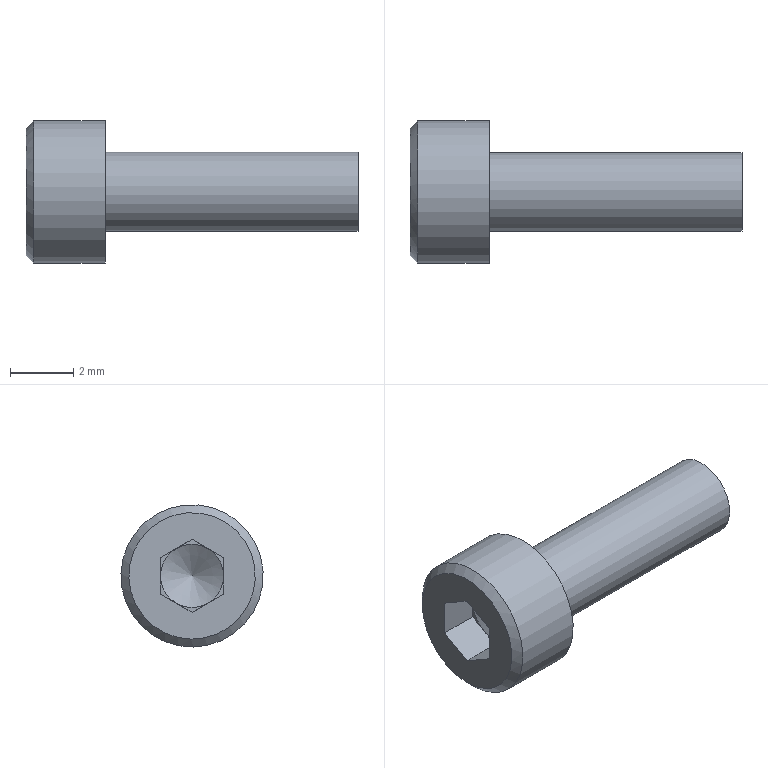Part | NX | features NEZI_5003_022_GCJC20-BL-6-8 2 | 1 solid | 19 faces | box 10.5 x 4.5 x 4.5 mm | volume 73.646 mm3 | plane 15 | cone 2 | cylinder 2 | commonest cylinder face diameters 2.5 x1 4.5 x1
STEP:
#1=CARTESIAN_POINT('',(-221.975,-582.6,-104.577));
#2=VERTEX_POINT('',#1);
#3=CARTESIAN_POINT('',(-221.975,-583.6,-105.155));
#4=VERTEX_POINT('',#3);
#5=CARTESIAN_POINT('',(-221.975,-582.6,-104.577));
#6=DIRECTION('',(0.,-0.866,-0.5));
#7=VECTOR('',#6,1000.);
#8=LINE('',#5,#7);
#9=EDGE_CURVE('',#2,#4,#8,.T.);
#10=ORIENTED_EDGE('',*,*,#9,.F.);
#11=CARTESIAN_POINT('',(-221.975,-582.6,-103.423));
#12=VERTEX_POINT('',#11);
#13=CARTESIAN_POINT('',(-221.975,-582.6,-103.423));
#14=DIRECTION('',(0.,0.,-1.));
#15=VECTOR('',#14,1000.);
#16=LINE('',#13,#15);
#17=EDGE_CURVE('',#12,#2,#16,.T.);
#18=ORIENTED_EDGE('',*,*,#17,.F.);
#19=CARTESIAN_POINT('',(-221.975,-583.6,-102.845));
#20=VERTEX_POINT('',#19);
#21=CARTESIAN_POINT('',(-221.975,-583.6,-102.845));
#22=DIRECTION('',(0.,0.866,-0.5));
#23=VECTOR('',#22,1000.);
#24=LINE('',#21,#23);
#25=EDGE_CURVE('',#20,#12,#24,.T.);
#26=ORIENTED_EDGE('',*,*,#25,.F.);
#27=CARTESIAN_POINT('',(-221.975,-584.6,-103.423));
#28=VERTEX_POINT('',#27);
#29=CARTESIAN_POINT('',(-221.975,-584.6,-103.423));
#30=DIRECTION('',(0.,0.866,0.5));
#31=VECTOR('',#30,1000.);
#32=LINE('',#29,#31);
#33=EDGE_CURVE('',#28,#20,#32,.T.);
#34=ORIENTED_EDGE('',*,*,#33,.F.);
#35=CARTESIAN_POINT('',(-221.975,-584.6,-104.577));
#36=VERTEX_POINT('',#35);
#37=CARTESIAN_POINT('',(-221.975,-584.6,-104.577));
#38=DIRECTION('',(0.,0.,1.));
#39=VECTOR('',#38,1000.);
#40=LINE('',#37,#39);
#41=EDGE_CURVE('',#36,#28,#40,.T.);
#42=ORIENTED_EDGE('',*,*,#41,.F.);
#43=CARTESIAN_POINT('',(-221.975,-583.6,-105.155));
#44=DIRECTION('',(0.,-0.866,0.5));
#45=VECTOR('',#44,1000.);
#46=LINE('',#43,#45);
#47=EDGE_CURVE('',#4,#36,#46,.T.);
#48=ORIENTED_EDGE('',*,*,#47,.F.);
#49=EDGE_LOOP('',(#10,#18,#26,#34,#42,#48));
#50=FACE_BOUND('',#49,.T.);
#51=CARTESIAN_POINT('',(-221.975,-582.6,-102.268));
#52=VERTEX_POINT('',#51);
#53=CARTESIAN_POINT('',(-221.975,-583.6,-104.));
#54=DIRECTION('',(-1.,0.,0.));
#55=DIRECTION('',(0.,0.5,0.866));
#56=AXIS2_PLACEMENT_3D('',#53,#54,#55);
#57=CIRCLE('',#56,2.);
#58=EDGE_CURVE('',#52,#52,#57,.T.);
#59=ORIENTED_EDGE('',*,*,#58,.T.);
#60=EDGE_LOOP('',(#59));
#61=FACE_BOUND('',#60,.T.);
#62=CARTESIAN_POINT('',(-221.975,-583.6,-104.));
#63=DIRECTION('',(1.,0.,0.));
#64=DIRECTION('',(0.,-0.5,-0.866));
#65=AXIS2_PLACEMENT_3D('',#62,#63,#64);
#66=PLANE('',#65);
#67=ADVANCED_FACE('',(#50,#61),#66,.F.);
#68=ORIENTED_EDGE('',*,*,#58,.F.);
#69=EDGE_LOOP('',(#68));
#70=FACE_BOUND('',#69,.T.);
#71=CARTESIAN_POINT('',(-221.725,-582.475,-102.051));
#72=VERTEX_POINT('',#71);
#73=CARTESIAN_POINT('',(-221.725,-583.6,-104.));
#74=DIRECTION('',(-1.,0.,0.));
#75=DIRECTION('',(0.,0.5,0.866));
#76=AXIS2_PLACEMENT_3D('',#73,#74,#75);
#77=CIRCLE('',#76,2.25);
#78=EDGE_CURVE('',#72,#72,#77,.T.);
#79=ORIENTED_EDGE('',*,*,#78,.T.);
#80=EDGE_LOOP('',(#79));
#81=FACE_BOUND('',#80,.T.);
#82=CARTESIAN_POINT('',(-221.725,-583.6,-104.));
#83=DIRECTION('',(1.,0.,0.));
#84=DIRECTION('',(0.,-0.5,-0.866));
#85=AXIS2_PLACEMENT_3D('',#82,#83,#84);
#86=CONICAL_SURFACE('',#85,2.25,0.7854);
#87=ADVANCED_FACE('',(#70,#81),#86,.T.);
#88=ORIENTED_EDGE('',*,*,#78,.F.);
#89=EDGE_LOOP('',(#88));
#90=FACE_BOUND('',#89,.T.);
#91=CARTESIAN_POINT('',(-219.475,-582.475,-102.051));
#92=VERTEX_POINT('',#91);
#93=CARTESIAN_POINT('',(-219.475,-583.6,-104.));
#94=DIRECTION('',(-1.,0.,0.));
#95=DIRECTION('',(0.,0.5,0.866));
#96=AXIS2_PLACEMENT_3D('',#93,#94,#95);
#97=CIRCLE('',#96,2.25);
#98=EDGE_CURVE('',#92,#92,#97,.T.);
#99=ORIENTED_EDGE('',*,*,#98,.T.);
#100=EDGE_LOOP('',(#99));
#101=FACE_BOUND('',#100,.T.);
#102=CARTESIAN_POINT('',(-222.5,-583.6,-104.));
#103=DIRECTION('',(-1.,0.,0.));
#104=DIRECTION('',(0.,0.5,0.866));
#105=AXIS2_PLACEMENT_3D('',#102,#103,#104);
#106=CYLINDRICAL_SURFACE('',#105,2.25);
#107=ADVANCED_FACE('',(#90,#101),#106,.T.);
#108=ORIENTED_EDGE('',*,*,#98,.F.);
#109=EDGE_LOOP('',(#108));
#110=FACE_BOUND('',#109,.T.);
#111=CARTESIAN_POINT('',(-219.475,-582.975,-102.917));
#112=VERTEX_POINT('',#111);
#113=CARTESIAN_POINT('',(-219.475,-583.6,-104.));
#114=DIRECTION('',(-1.,0.,0.));
#115=DIRECTION('',(0.,0.5,0.866));
#116=AXIS2_PLACEMENT_3D('',#113,#114,#115);
#117=CIRCLE('',#116,1.25);
#118=EDGE_CURVE('',#112,#112,#117,.T.);
#119=ORIENTED_EDGE('',*,*,#118,.T.);
#120=EDGE_LOOP('',(#119));
#121=FACE_BOUND('',#120,.T.);
#122=CARTESIAN_POINT('',(-219.475,-581.651,-105.125));
#123=DIRECTION('',(-1.,0.,0.));
#124=DIRECTION('',(0.,0.5,0.866));
#125=AXIS2_PLACEMENT_3D('',#122,#123,#124);
#126=PLANE('',#125);
#127=ADVANCED_FACE('',(#110,#121),#126,.F.);
#128=ORIENTED_EDGE('',*,*,#118,.F.);
#129=EDGE_LOOP('',(#128));
#130=FACE_BOUND('',#129,.T.);
#131=CARTESIAN_POINT('',(-211.475,-582.975,-102.917));
#132=VERTEX_POINT('',#131);
#133=CARTESIAN_POINT('',(-211.475,-583.6,-104.));
#134=DIRECTION('',(-1.,0.,0.));
#135=DIRECTION('',(0.,0.5,0.866));
#136=AXIS2_PLACEMENT_3D('',#133,#134,#135);
#137=CIRCLE('',#136,1.25);
#138=EDGE_CURVE('',#132,#132,#137,.T.);
#139=ORIENTED_EDGE('',*,*,#138,.T.);
#140=EDGE_LOOP('',(#139));
#141=FACE_BOUND('',#140,.T.);
#142=CARTESIAN_POINT('',(-222.5,-583.6,-104.));
#143=DIRECTION('',(-1.,0.,0.));
#144=DIRECTION('',(0.,0.5,0.866));
#145=AXIS2_PLACEMENT_3D('',#142,#143,#144);
#146=CYLINDRICAL_SURFACE('',#145,1.25);
#147=ADVANCED_FACE('',(#130,#141),#146,.T.);
#148=ORIENTED_EDGE('',*,*,#138,.F.);
#149=EDGE_LOOP('',(#148));
#150=FACE_BOUND('',#149,.T.);
#151=CARTESIAN_POINT('',(-211.475,-582.517,-104.625));
#152=DIRECTION('',(-1.,0.,0.));
#153=DIRECTION('',(0.,0.5,0.866));
#154=AXIS2_PLACEMENT_3D('',#151,#152,#153);
#155=PLANE('',#154);
#156=ADVANCED_FACE('',(#150),#155,.F.);
#157=ORIENTED_EDGE('',*,*,#17,.T.);
#158=CARTESIAN_POINT('',(-220.725,-582.6,-104.577));
#159=VERTEX_POINT('',#158);
#160=CARTESIAN_POINT('',(-220.725,-582.6,-104.577));
#161=DIRECTION('',(-1.,0.,0.));
#162=VECTOR('',#161,1000.);
#163=LINE('',#160,#162);
#164=EDGE_CURVE('',#159,#2,#163,.T.);
#165=ORIENTED_EDGE('',*,*,#164,.F.);
#166=CARTESIAN_POINT('',(-220.725,-582.6,-104.));
#167=VERTEX_POINT('',#166);
#168=CARTESIAN_POINT('',(-220.725,-582.6,-103.423));
#169=DIRECTION('',(0.,0.,-1.));
#170=VECTOR('',#169,1000.);
#171=LINE('',#168,#170);
#172=EDGE_CURVE('',#167,#159,#171,.T.);
#173=ORIENTED_EDGE('',*,*,#172,.F.);
#174=CARTESIAN_POINT('',(-220.725,-582.6,-103.423));
#175=VERTEX_POINT('',#174);
#176=CARTESIAN_POINT('',(-220.725,-582.6,-103.423));
#177=DIRECTION('',(0.,0.,-1.));
#178=VECTOR('',#177,1000.);
#179=LINE('',#176,#178);
#180=EDGE_CURVE('',#175,#167,#179,.T.);
#181=ORIENTED_EDGE('',*,*,#180,.F.);
#182=CARTESIAN_POINT('',(-220.725,-582.6,-103.423));
#183=DIRECTION('',(-1.,0.,0.));
#184=VECTOR('',#183,1000.);
#185=LINE('',#182,#184);
#186=EDGE_CURVE('',#175,#12,#185,.T.);
#187=ORIENTED_EDGE('',*,*,#186,.T.);
#188=EDGE_LOOP('',(#157,#165,#173,#181,#187));
#189=FACE_BOUND('',#188,.T.);
#190=CARTESIAN_POINT('',(-220.725,-582.6,-103.423));
#191=DIRECTION('',(0.,1.,0.));
#192=DIRECTION('',(0.,0.,1.));
#193=AXIS2_PLACEMENT_3D('',#190,#191,#192);
#194=PLANE('',#193);
#195=ADVANCED_FACE('',(#189),#194,.F.);
#196=ORIENTED_EDGE('',*,*,#25,.T.);
#197=ORIENTED_EDGE('',*,*,#186,.F.);
#198=CARTESIAN_POINT('',(-220.725,-583.1,-103.134));
#199=VERTEX_POINT('',#198);
#200=CARTESIAN_POINT('',(-220.725,-583.6,-102.845));
#201=DIRECTION('',(0.,0.866,-0.5));
#202=VECTOR('',#201,1000.);
#203=LINE('',#200,#202);
#204=EDGE_CURVE('',#199,#175,#203,.T.);
#205=ORIENTED_EDGE('',*,*,#204,.F.);
#206=CARTESIAN_POINT('',(-220.725,-583.6,-102.845));
#207=VERTEX_POINT('',#206);
#208=CARTESIAN_POINT('',(-220.725,-583.6,-102.845));
#209=DIRECTION('',(0.,0.866,-0.5));
#210=VECTOR('',#209,1000.);
#211=LINE('',#208,#210);
#212=EDGE_CURVE('',#207,#199,#211,.T.);
#213=ORIENTED_EDGE('',*,*,#212,.F.);
#214=CARTESIAN_POINT('',(-220.725,-583.6,-102.845));
#215=DIRECTION('',(-1.,0.,0.));
#216=VECTOR('',#215,1000.);
#217=LINE('',#214,#216);
#218=EDGE_CURVE('',#207,#20,#217,.T.);
#219=ORIENTED_EDGE('',*,*,#218,.T.);
#220=EDGE_LOOP('',(#196,#197,#205,#213,#219));
#221=FACE_BOUND('',#220,.T.);
#222=CARTESIAN_POINT('',(-220.725,-583.6,-102.845));
#223=DIRECTION('',(0.,0.5,0.866));
#224=DIRECTION('',(1.,0.,0.));
#225=AXIS2_PLACEMENT_3D('',#222,#223,#224);
#226=PLANE('',#225);
#227=ADVANCED_FACE('',(#221),#226,.F.);
#228=ORIENTED_EDGE('',*,*,#33,.T.);
#229=ORIENTED_EDGE('',*,*,#218,.F.);
#230=CARTESIAN_POINT('',(-220.725,-584.1,-103.134));
#231=VERTEX_POINT('',#230);
#232=CARTESIAN_POINT('',(-220.725,-584.6,-103.423));
#233=DIRECTION('',(0.,0.866,0.5));
#234=VECTOR('',#233,1000.);
#235=LINE('',#232,#234);
#236=EDGE_CURVE('',#231,#207,#235,.T.);
#237=ORIENTED_EDGE('',*,*,#236,.F.);
#238=CARTESIAN_POINT('',(-220.725,-584.6,-103.423));
#239=VERTEX_POINT('',#238);
#240=CARTESIAN_POINT('',(-220.725,-584.6,-103.423));
#241=DIRECTION('',(0.,0.866,0.5));
#242=VECTOR('',#241,1000.);
#243=LINE('',#240,#242);
#244=EDGE_CURVE('',#239,#231,#243,.T.);
#245=ORIENTED_EDGE('',*,*,#244,.F.);
#246=CARTESIAN_POINT('',(-220.725,-584.6,-103.423));
#247=DIRECTION('',(-1.,0.,0.));
#248=VECTOR('',#247,1000.);
#249=LINE('',#246,#248);
#250=EDGE_CURVE('',#239,#28,#249,.T.);
#251=ORIENTED_EDGE('',*,*,#250,.T.);
#252=EDGE_LOOP('',(#228,#229,#237,#245,#251));
#253=FACE_BOUND('',#252,.T.);
#254=CARTESIAN_POINT('',(-220.725,-584.6,-103.423));
#255=DIRECTION('',(0.,-0.5,0.866));
#256=DIRECTION('',(0.,-0.866,-0.5));
#257=AXIS2_PLACEMENT_3D('',#254,#255,#256);
#258=PLANE('',#257);
#259=ADVANCED_FACE('',(#253),#258,.F.);
#260=ORIENTED_EDGE('',*,*,#41,.T.);
#261=ORIENTED_EDGE('',*,*,#250,.F.);
#262=CARTESIAN_POINT('',(-220.725,-584.6,-104.));
#263=VERTEX_POINT('',#262);
#264=CARTESIAN_POINT('',(-220.725,-584.6,-104.577));
#265=DIRECTION('',(0.,0.,1.));
#266=VECTOR('',#265,1000.);
#267=LINE('',#264,#266);
#268=EDGE_CURVE('',#263,#239,#267,.T.);
#269=ORIENTED_EDGE('',*,*,#268,.F.);
#270=CARTESIAN_POINT('',(-220.725,-584.6,-104.577));
#271=VERTEX_POINT('',#270);
#272=CARTESIAN_POINT('',(-220.725,-584.6,-104.577));
#273=DIRECTION('',(0.,0.,1.));
#274=VECTOR('',#273,1000.);
#275=LINE('',#272,#274);
#276=EDGE_CURVE('',#271,#263,#275,.T.);
#277=ORIENTED_EDGE('',*,*,#276,.F.);
#278=CARTESIAN_POINT('',(-220.725,-584.6,-104.577));
#279=DIRECTION('',(-1.,0.,0.));
#280=VECTOR('',#279,1000.);
#281=LINE('',#278,#280);
#282=EDGE_CURVE('',#271,#36,#281,.T.);
#283=ORIENTED_EDGE('',*,*,#282,.T.);
#284=EDGE_LOOP('',(#260,#261,#269,#277,#283));
#285=FACE_BOUND('',#284,.T.);
#286=CARTESIAN_POINT('',(-220.725,-584.6,-104.577));
#287=DIRECTION('',(0.,-1.,0.));
#288=DIRECTION('',(0.,0.,-1.));
#289=AXIS2_PLACEMENT_3D('',#286,#287,#288);
#290=PLANE('',#289);
#291=ADVANCED_FACE('',(#285),#290,.F.);
#292=ORIENTED_EDGE('',*,*,#47,.T.);
#293=ORIENTED_EDGE('',*,*,#282,.F.);
#294=CARTESIAN_POINT('',(-220.725,-584.1,-104.866));
#295=VERTEX_POINT('',#294);
#296=CARTESIAN_POINT('',(-220.725,-583.6,-105.155));
#297=DIRECTION('',(0.,-0.866,0.5));
#298=VECTOR('',#297,1000.);
#299=LINE('',#296,#298);
#300=EDGE_CURVE('',#295,#271,#299,.T.);
#301=ORIENTED_EDGE('',*,*,#300,.F.);
#302=CARTESIAN_POINT('',(-220.725,-583.6,-105.155));
#303=VERTEX_POINT('',#302);
#304=CARTESIAN_POINT('',(-220.725,-583.6,-105.155));
#305=DIRECTION('',(0.,-0.866,0.5));
#306=VECTOR('',#305,1000.);
#307=LINE('',#304,#306);
#308=EDGE_CURVE('',#303,#295,#307,.T.);
#309=ORIENTED_EDGE('',*,*,#308,.F.);
#310=CARTESIAN_POINT('',(-220.725,-583.6,-105.155));
#311=DIRECTION('',(-1.,0.,0.));
#312=VECTOR('',#311,1000.);
#313=LINE('',#310,#312);
#314=EDGE_CURVE('',#303,#4,#313,.T.);
#315=ORIENTED_EDGE('',*,*,#314,.T.);
#316=EDGE_LOOP('',(#292,#293,#301,#309,#315));
#317=FACE_BOUND('',#316,.T.);
#318=CARTESIAN_POINT('',(-220.725,-583.6,-105.155));
#319=DIRECTION('',(0.,-0.5,-0.866));
#320=DIRECTION('',(-1.,0.,0.));
#321=AXIS2_PLACEMENT_3D('',#318,#319,#320);
#322=PLANE('',#321);
#323=ADVANCED_FACE('',(#317),#322,.F.);
#324=ORIENTED_EDGE('',*,*,#9,.T.);
#325=ORIENTED_EDGE('',*,*,#314,.F.);
#326=CARTESIAN_POINT('',(-220.725,-583.1,-104.866));
#327=VERTEX_POINT('',#326);
#328=CARTESIAN_POINT('',(-220.725,-582.6,-104.577));
#329=DIRECTION('',(0.,-0.866,-0.5));
#330=VECTOR('',#329,1000.);
#331=LINE('',#328,#330);
#332=EDGE_CURVE('',#327,#303,#331,.T.);
#333=ORIENTED_EDGE('',*,*,#332,.F.);
#334=CARTESIAN_POINT('',(-220.725,-582.6,-104.577));
#335=DIRECTION('',(0.,-0.866,-0.5));
#336=VECTOR('',#335,1000.);
#337=LINE('',#334,#336);
#338=EDGE_CURVE('',#159,#327,#337,.T.);
#339=ORIENTED_EDGE('',*,*,#338,.F.);
#340=ORIENTED_EDGE('',*,*,#164,.T.);
#341=EDGE_LOOP('',(#324,#325,#333,#339,#340));
#342=FACE_BOUND('',#341,.T.);
#343=CARTESIAN_POINT('',(-220.725,-582.6,-104.577));
#344=DIRECTION('',(0.,0.5,-0.866));
#345=DIRECTION('',(0.,0.866,0.5));
#346=AXIS2_PLACEMENT_3D('',#343,#344,#345);
#347=PLANE('',#346);
#348=ADVANCED_FACE('',(#342),#347,.F.);
#349=CARTESIAN_POINT('',(-220.725,-583.6,-104.));
#350=DIRECTION('',(-1.,0.,0.));
#351=DIRECTION('',(0.,0.5,0.866));
#352=AXIS2_PLACEMENT_3D('',#349,#350,#351);
#353=CIRCLE('',#352,1.);
#354=EDGE_CURVE('',#231,#199,#353,.T.);
#355=ORIENTED_EDGE('',*,*,#354,.F.);
#356=ORIENTED_EDGE('',*,*,#236,.T.);
#357=ORIENTED_EDGE('',*,*,#212,.T.);
#358=EDGE_LOOP('',(#355,#356,#357));
#359=FACE_BOUND('',#358,.T.);
#360=CARTESIAN_POINT('',(-220.725,-583.6,-104.));
#361=DIRECTION('',(-1.,0.,0.));
#362=DIRECTION('',(0.,0.5,0.866));
#363=AXIS2_PLACEMENT_3D('',#360,#361,#362);
#364=PLANE('',#363);
#365=ADVANCED_FACE('',(#359),#364,.T.);
#366=CARTESIAN_POINT('',(-220.725,-583.6,-104.));
#367=DIRECTION('',(-1.,0.,0.));
#368=DIRECTION('',(0.,0.5,0.866));
#369=AXIS2_PLACEMENT_3D('',#366,#367,#368);
#370=CIRCLE('',#369,1.);
#371=EDGE_CURVE('',#263,#231,#370,.T.);
#372=ORIENTED_EDGE('',*,*,#371,.F.);
#373=ORIENTED_EDGE('',*,*,#268,.T.);
#374=ORIENTED_EDGE('',*,*,#244,.T.);
#375=EDGE_LOOP('',(#372,#373,#374));
#376=FACE_BOUND('',#375,.T.);
#377=CARTESIAN_POINT('',(-220.725,-583.6,-104.));
#378=DIRECTION('',(-1.,0.,0.));
#379=DIRECTION('',(0.,0.5,0.866));
#380=AXIS2_PLACEMENT_3D('',#377,#378,#379);
#381=PLANE('',#380);
#382=ADVANCED_FACE('',(#376),#381,.T.);
#383=CARTESIAN_POINT('',(-220.725,-583.6,-104.));
#384=DIRECTION('',(-1.,0.,0.));
#385=DIRECTION('',(0.,0.5,0.866));
#386=AXIS2_PLACEMENT_3D('',#383,#384,#385);
#387=CIRCLE('',#386,1.);
#388=EDGE_CURVE('',#295,#263,#387,.T.);
#389=ORIENTED_EDGE('',*,*,#388,.F.);
#390=ORIENTED_EDGE('',*,*,#300,.T.);
#391=ORIENTED_EDGE('',*,*,#276,.T.);
#392=EDGE_LOOP('',(#389,#390,#391));
#393=FACE_BOUND('',#392,.T.);
#394=CARTESIAN_POINT('',(-220.725,-583.6,-104.));
#395=DIRECTION('',(-1.,0.,0.));
#396=DIRECTION('',(0.,0.5,0.866));
#397=AXIS2_PLACEMENT_3D('',#394,#395,#396);
#398=PLANE('',#397);
#399=ADVANCED_FACE('',(#393),#398,.T.);
#400=CARTESIAN_POINT('',(-220.725,-583.6,-104.));
#401=DIRECTION('',(-1.,0.,0.));
#402=DIRECTION('',(0.,0.5,0.866));
#403=AXIS2_PLACEMENT_3D('',#400,#401,#402);
#404=CIRCLE('',#403,1.);
#405=EDGE_CURVE('',#327,#295,#404,.T.);
#406=ORIENTED_EDGE('',*,*,#405,.F.);
#407=ORIENTED_EDGE('',*,*,#332,.T.);
#408=ORIENTED_EDGE('',*,*,#308,.T.);
#409=EDGE_LOOP('',(#406,#407,#408));
#410=FACE_BOUND('',#409,.T.);
#411=CARTESIAN_POINT('',(-220.725,-583.6,-104.));
#412=DIRECTION('',(-1.,0.,0.));
#413=DIRECTION('',(0.,0.5,0.866));
#414=AXIS2_PLACEMENT_3D('',#411,#412,#413);
#415=PLANE('',#414);
#416=ADVANCED_FACE('',(#410),#415,.T.);
#417=CARTESIAN_POINT('',(-220.725,-583.6,-104.));
#418=DIRECTION('',(-1.,0.,0.));
#419=DIRECTION('',(0.,0.5,0.866));
#420=AXIS2_PLACEMENT_3D('',#417,#418,#419);
#421=CIRCLE('',#420,1.);
#422=EDGE_CURVE('',#167,#327,#421,.T.);
#423=ORIENTED_EDGE('',*,*,#422,.F.);
#424=ORIENTED_EDGE('',*,*,#172,.T.);
#425=ORIENTED_EDGE('',*,*,#338,.T.);
#426=EDGE_LOOP('',(#423,#424,#425));
#427=FACE_BOUND('',#426,.T.);
#428=CARTESIAN_POINT('',(-220.725,-583.6,-104.));
#429=DIRECTION('',(-1.,0.,0.));
#430=DIRECTION('',(0.,0.5,0.866));
#431=AXIS2_PLACEMENT_3D('',#428,#429,#430);
#432=PLANE('',#431);
#433=ADVANCED_FACE('',(#427),#432,.T.);
#434=CARTESIAN_POINT('',(-220.725,-583.6,-104.));
#435=DIRECTION('',(-1.,0.,0.));
#436=DIRECTION('',(0.,0.5,0.866));
#437=AXIS2_PLACEMENT_3D('',#434,#435,#436);
#438=CIRCLE('',#437,1.);
#439=EDGE_CURVE('',#199,#167,#438,.T.);
#440=ORIENTED_EDGE('',*,*,#439,.F.);
#441=ORIENTED_EDGE('',*,*,#204,.T.);
#442=ORIENTED_EDGE('',*,*,#180,.T.);
#443=EDGE_LOOP('',(#440,#441,#442));
#444=FACE_BOUND('',#443,.T.);
#445=CARTESIAN_POINT('',(-220.725,-583.6,-104.));
#446=DIRECTION('',(-1.,0.,0.));
#447=DIRECTION('',(0.,0.5,0.866));
#448=AXIS2_PLACEMENT_3D('',#445,#446,#447);
#449=PLANE('',#448);
#450=ADVANCED_FACE('',(#444),#449,.T.);
#451=CARTESIAN_POINT('',(-220.124,-583.6,-104.));
#452=VERTEX_POINT('',#451);
#453=VERTEX_LOOP('',#452);
#454=FACE_BOUND('',#453,.T.);
#455=ORIENTED_EDGE('',*,*,#439,.T.);
#456=ORIENTED_EDGE('',*,*,#422,.T.);
#457=ORIENTED_EDGE('',*,*,#405,.T.);
#458=ORIENTED_EDGE('',*,*,#388,.T.);
#459=ORIENTED_EDGE('',*,*,#371,.T.);
#460=ORIENTED_EDGE('',*,*,#354,.T.);
#461=EDGE_LOOP('',(#455,#456,#457,#458,#459,#460));
#462=FACE_BOUND('',#461,.T.);
#463=CARTESIAN_POINT('',(-220.725,-583.6,-104.));
#464=DIRECTION('',(-1.,0.,0.));
#465=DIRECTION('',(0.,0.5,0.866));
#466=AXIS2_PLACEMENT_3D('',#463,#464,#465);
#467=CONICAL_SURFACE('',#466,1.,1.03);
#468=ADVANCED_FACE('',(#454,#462),#467,.F.);
#469=CLOSED_SHELL('',(#67,#87,#107,#127,#147,#156,#195,#227,#259,#291,#323,#348,#365,#382,#399,#416,#433,#450,#468));
#470=MANIFOLD_SOLID_BREP('',#469);
#471=(LENGTH_UNIT()NAMED_UNIT(*)SI_UNIT(.MILLI.,.METRE.));
#472=UNCERTAINTY_MEASURE_WITH_UNIT(LENGTH_MEASURE(0.00001),#471,'','');
#473=(NAMED_UNIT(*)PLANE_ANGLE_UNIT()SI_UNIT($,.RADIAN.));
#474=(NAMED_UNIT(*)SI_UNIT($,.STERADIAN.)SOLID_ANGLE_UNIT());
#475=(GEOMETRIC_REPRESENTATION_CONTEXT(3)GLOBAL_UNCERTAINTY_ASSIGNED_CONTEXT((#472))GLOBAL_UNIT_ASSIGNED_CONTEXT((#471,#473,#474))REPRESENTATION_CONTEXT('',''));
#476=ADVANCED_BREP_SHAPE_REPRESENTATION('',(#470),#475);